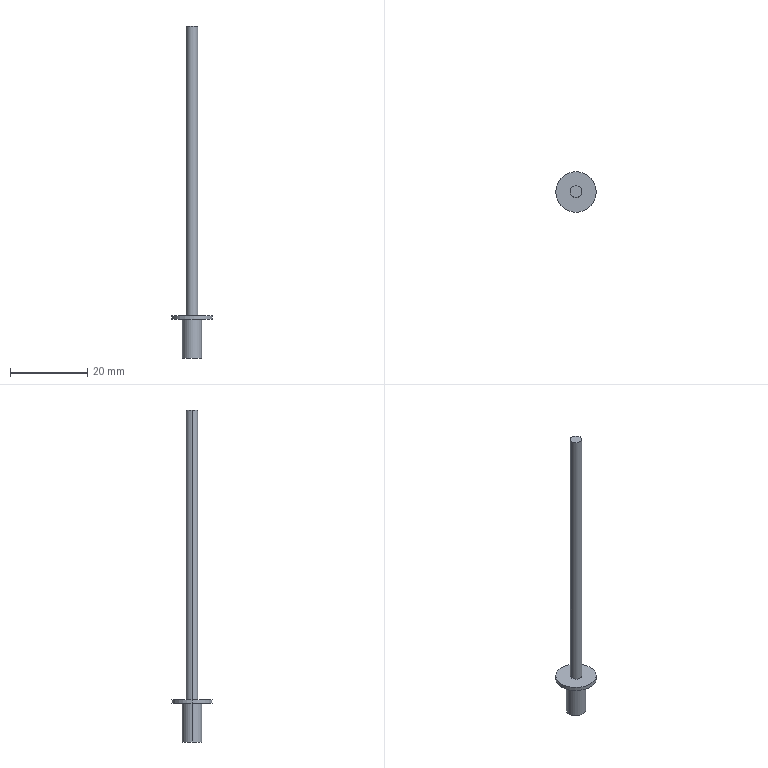Part | Creo | 1 solid | 10 faces | box 10.5 x 10.5 x 86 mm | volume 813.083 mm3 | cylinder 6 | plane 4 | commonest cylinder face diameters 3 x2 5 x2 10.5 x2
STEP:
#1=CARTESIAN_POINT('',(0.,0.,0.));
#2=DIRECTION('',(0.,0.,1.));
#3=DIRECTION('',(1.,0.,0.));
#4=AXIS2_PLACEMENT_3D('',#1,#2,#3);
#5=CARTESIAN_POINT('',(35.5,79.,-54.09));
#6=VERTEX_POINT('',#5);
#7=CARTESIAN_POINT('',(38.5,79.,-54.09));
#8=VERTEX_POINT('',#7);
#9=CARTESIAN_POINT('',(37.,79.,-54.09));
#10=DIRECTION('',(0.,0.,-1.));
#11=DIRECTION('',(-1.,0.,0.));
#12=AXIS2_PLACEMENT_3D('',#9,#10,#11);
#13=CIRCLE('',#12,1.5);
#14=EDGE_CURVE('',#6,#8,#13,.T.);
#15=ORIENTED_EDGE('',*,*,#14,.T.);
#16=CARTESIAN_POINT('',(38.5,79.,20.91));
#17=VERTEX_POINT('',#16);
#18=CARTESIAN_POINT('',(38.5,79.,20.91));
#19=DIRECTION('',(0.,0.,-1.));
#20=VECTOR('',#19,75.);
#21=LINE('',#18,#20);
#22=EDGE_CURVE('',#17,#8,#21,.T.);
#23=ORIENTED_EDGE('',*,*,#22,.F.);
#24=CARTESIAN_POINT('',(35.5,79.,20.91));
#25=VERTEX_POINT('',#24);
#26=CARTESIAN_POINT('',(37.,79.,20.91));
#27=DIRECTION('',(0.,0.,1.));
#28=DIRECTION('',(1.,0.,0.));
#29=AXIS2_PLACEMENT_3D('',#26,#27,#28);
#30=CIRCLE('',#29,1.5);
#31=EDGE_CURVE('',#17,#25,#30,.T.);
#32=ORIENTED_EDGE('',*,*,#31,.T.);
#33=CARTESIAN_POINT('',(35.5,79.,20.91));
#34=DIRECTION('',(0.,0.,-1.));
#35=VECTOR('',#34,75.);
#36=LINE('',#33,#35);
#37=EDGE_CURVE('',#25,#6,#36,.T.);
#38=ORIENTED_EDGE('',*,*,#37,.T.);
#39=EDGE_LOOP('',(#15,#23,#32,#38));
#40=FACE_OUTER_BOUND('',#39,.F.);
#41=CARTESIAN_POINT('',(37.,79.,20.91));
#42=DIRECTION('',(0.,0.,-1.));
#43=DIRECTION('',(-1.,0.,0.));
#44=AXIS2_PLACEMENT_3D('',#41,#42,#43);
#45=CYLINDRICAL_SURFACE('',#44,1.5);
#46=ADVANCED_FACE('',(#40),#45,.T.);
#47=CARTESIAN_POINT('',(31.75,79.,-54.09));
#48=VERTEX_POINT('',#47);
#49=CARTESIAN_POINT('',(42.25,79.,-54.09));
#50=VERTEX_POINT('',#49);
#51=CARTESIAN_POINT('',(37.,79.,-54.09));
#52=DIRECTION('',(0.,0.,1.));
#53=DIRECTION('',(-1.,0.,0.));
#54=AXIS2_PLACEMENT_3D('',#51,#52,#53);
#55=CIRCLE('',#54,5.25);
#56=EDGE_CURVE('',#48,#50,#55,.T.);
#57=ORIENTED_EDGE('',*,*,#56,.F.);
#58=CARTESIAN_POINT('',(37.,79.,-54.09));
#59=DIRECTION('',(0.,0.,1.));
#60=DIRECTION('',(1.,0.,0.));
#61=AXIS2_PLACEMENT_3D('',#58,#59,#60);
#62=CIRCLE('',#61,5.25);
#63=EDGE_CURVE('',#50,#48,#62,.T.);
#64=ORIENTED_EDGE('',*,*,#63,.F.);
#65=EDGE_LOOP('',(#57,#64));
#66=FACE_OUTER_BOUND('',#65,.F.);
#67=ORIENTED_EDGE('',*,*,#14,.F.);
#68=CARTESIAN_POINT('',(37.,79.,-54.09));
#69=DIRECTION('',(0.,0.,-1.));
#70=DIRECTION('',(1.,0.,0.));
#71=AXIS2_PLACEMENT_3D('',#68,#69,#70);
#72=CIRCLE('',#71,1.5);
#73=EDGE_CURVE('',#8,#6,#72,.T.);
#74=ORIENTED_EDGE('',*,*,#73,.F.);
#75=EDGE_LOOP('',(#67,#74));
#76=FACE_BOUND('',#75,.F.);
#77=CARTESIAN_POINT('',(0.,0.,-54.09));
#78=DIRECTION('',(0.,0.,-1.));
#79=DIRECTION('',(-1.,0.,0.));
#80=AXIS2_PLACEMENT_3D('',#77,#78,#79);
#81=PLANE('',#80);
#82=ADVANCED_FACE('',(#66,#76),#81,.F.);
#83=ORIENTED_EDGE('',*,*,#73,.T.);
#84=ORIENTED_EDGE('',*,*,#37,.F.);
#85=CARTESIAN_POINT('',(37.,79.,20.91));
#86=DIRECTION('',(0.,0.,1.));
#87=DIRECTION('',(-1.,0.,0.));
#88=AXIS2_PLACEMENT_3D('',#85,#86,#87);
#89=CIRCLE('',#88,1.5);
#90=EDGE_CURVE('',#25,#17,#89,.T.);
#91=ORIENTED_EDGE('',*,*,#90,.T.);
#92=ORIENTED_EDGE('',*,*,#22,.T.);
#93=EDGE_LOOP('',(#83,#84,#91,#92));
#94=FACE_OUTER_BOUND('',#93,.F.);
#95=CARTESIAN_POINT('',(37.,79.,20.91));
#96=DIRECTION('',(0.,0.,-1.));
#97=DIRECTION('',(-1.,0.,0.));
#98=AXIS2_PLACEMENT_3D('',#95,#96,#97);
#99=CYLINDRICAL_SURFACE('',#98,1.5);
#100=ADVANCED_FACE('',(#94),#99,.T.);
#101=ORIENTED_EDGE('',*,*,#90,.F.);
#102=ORIENTED_EDGE('',*,*,#31,.F.);
#103=EDGE_LOOP('',(#101,#102));
#104=FACE_OUTER_BOUND('',#103,.F.);
#105=CARTESIAN_POINT('',(37.,79.,20.91));
#106=DIRECTION('',(0.,0.,-1.));
#107=DIRECTION('',(-1.,0.,0.));
#108=AXIS2_PLACEMENT_3D('',#105,#106,#107);
#109=PLANE('',#108);
#110=ADVANCED_FACE('',(#104),#109,.F.);
#111=ORIENTED_EDGE('',*,*,#56,.T.);
#112=CARTESIAN_POINT('',(42.25,79.,-55.09));
#113=VERTEX_POINT('',#112);
#114=CARTESIAN_POINT('',(42.25,79.,-55.09));
#115=DIRECTION('',(0.,0.,1.));
#116=VECTOR('',#115,1.);
#117=LINE('',#114,#116);
#118=EDGE_CURVE('',#113,#50,#117,.T.);
#119=ORIENTED_EDGE('',*,*,#118,.F.);
#120=CARTESIAN_POINT('',(31.75,79.,-55.09));
#121=VERTEX_POINT('',#120);
#122=CARTESIAN_POINT('',(37.,79.,-55.09));
#123=DIRECTION('',(0.,0.,-1.));
#124=DIRECTION('',(1.,0.,0.));
#125=AXIS2_PLACEMENT_3D('',#122,#123,#124);
#126=CIRCLE('',#125,5.25);
#127=EDGE_CURVE('',#113,#121,#126,.T.);
#128=ORIENTED_EDGE('',*,*,#127,.T.);
#129=CARTESIAN_POINT('',(31.75,79.,-55.09));
#130=DIRECTION('',(0.,0.,1.));
#131=VECTOR('',#130,1.);
#132=LINE('',#129,#131);
#133=EDGE_CURVE('',#121,#48,#132,.T.);
#134=ORIENTED_EDGE('',*,*,#133,.T.);
#135=EDGE_LOOP('',(#111,#119,#128,#134));
#136=FACE_OUTER_BOUND('',#135,.F.);
#137=CARTESIAN_POINT('',(37.,79.,-104.09));
#138=DIRECTION('',(0.,0.,1.));
#139=DIRECTION('',(1.,0.,0.));
#140=AXIS2_PLACEMENT_3D('',#137,#138,#139);
#141=CYLINDRICAL_SURFACE('',#140,5.25);
#142=ADVANCED_FACE('',(#136),#141,.T.);
#143=ORIENTED_EDGE('',*,*,#63,.T.);
#144=ORIENTED_EDGE('',*,*,#133,.F.);
#145=CARTESIAN_POINT('',(37.,79.,-55.09));
#146=DIRECTION('',(0.,0.,-1.));
#147=DIRECTION('',(-1.,0.,0.));
#148=AXIS2_PLACEMENT_3D('',#145,#146,#147);
#149=CIRCLE('',#148,5.25);
#150=EDGE_CURVE('',#121,#113,#149,.T.);
#151=ORIENTED_EDGE('',*,*,#150,.T.);
#152=ORIENTED_EDGE('',*,*,#118,.T.);
#153=EDGE_LOOP('',(#143,#144,#151,#152));
#154=FACE_OUTER_BOUND('',#153,.F.);
#155=CARTESIAN_POINT('',(37.,79.,-104.09));
#156=DIRECTION('',(0.,0.,1.));
#157=DIRECTION('',(1.,0.,0.));
#158=AXIS2_PLACEMENT_3D('',#155,#156,#157);
#159=CYLINDRICAL_SURFACE('',#158,5.25);
#160=ADVANCED_FACE('',(#154),#159,.T.);
#161=ORIENTED_EDGE('',*,*,#150,.F.);
#162=ORIENTED_EDGE('',*,*,#127,.F.);
#163=EDGE_LOOP('',(#161,#162));
#164=FACE_OUTER_BOUND('',#163,.F.);
#165=CARTESIAN_POINT('',(34.5,79.,-55.09));
#166=VERTEX_POINT('',#165);
#167=CARTESIAN_POINT('',(39.5,79.,-55.09));
#168=VERTEX_POINT('',#167);
#169=CARTESIAN_POINT('',(37.,79.,-55.09));
#170=DIRECTION('',(0.,0.,1.));
#171=DIRECTION('',(-1.,0.,0.));
#172=AXIS2_PLACEMENT_3D('',#169,#170,#171);
#173=CIRCLE('',#172,2.5);
#174=EDGE_CURVE('',#166,#168,#173,.T.);
#175=ORIENTED_EDGE('',*,*,#174,.F.);
#176=CARTESIAN_POINT('',(37.,79.,-55.09));
#177=DIRECTION('',(0.,0.,1.));
#178=DIRECTION('',(1.,0.,0.));
#179=AXIS2_PLACEMENT_3D('',#176,#177,#178);
#180=CIRCLE('',#179,2.5);
#181=EDGE_CURVE('',#168,#166,#180,.T.);
#182=ORIENTED_EDGE('',*,*,#181,.F.);
#183=EDGE_LOOP('',(#175,#182));
#184=FACE_BOUND('',#183,.F.);
#185=CARTESIAN_POINT('',(0.,0.,-55.09));
#186=DIRECTION('',(0.,0.,-1.));
#187=DIRECTION('',(-1.,0.,0.));
#188=AXIS2_PLACEMENT_3D('',#185,#186,#187);
#189=PLANE('',#188);
#190=ADVANCED_FACE('',(#164,#184),#189,.T.);
#191=CARTESIAN_POINT('',(39.5,79.,-65.09));
#192=VERTEX_POINT('',#191);
#193=CARTESIAN_POINT('',(34.5,79.,-65.09));
#194=VERTEX_POINT('',#193);
#195=CARTESIAN_POINT('',(37.,79.,-65.09));
#196=DIRECTION('',(0.,0.,-1.));
#197=DIRECTION('',(1.,0.,0.));
#198=AXIS2_PLACEMENT_3D('',#195,#196,#197);
#199=CIRCLE('',#198,2.5);
#200=EDGE_CURVE('',#192,#194,#199,.T.);
#201=ORIENTED_EDGE('',*,*,#200,.T.);
#202=CARTESIAN_POINT('',(34.5,79.,-55.09));
#203=DIRECTION('',(0.,0.,-1.));
#204=VECTOR('',#203,10.);
#205=LINE('',#202,#204);
#206=EDGE_CURVE('',#166,#194,#205,.T.);
#207=ORIENTED_EDGE('',*,*,#206,.F.);
#208=ORIENTED_EDGE('',*,*,#174,.T.);
#209=CARTESIAN_POINT('',(39.5,79.,-55.09));
#210=DIRECTION('',(0.,0.,-1.));
#211=VECTOR('',#210,10.);
#212=LINE('',#209,#211);
#213=EDGE_CURVE('',#168,#192,#212,.T.);
#214=ORIENTED_EDGE('',*,*,#213,.T.);
#215=EDGE_LOOP('',(#201,#207,#208,#214));
#216=FACE_OUTER_BOUND('',#215,.F.);
#217=CARTESIAN_POINT('',(37.,79.,-55.09));
#218=DIRECTION('',(0.,0.,-1.));
#219=DIRECTION('',(-1.,0.,0.));
#220=AXIS2_PLACEMENT_3D('',#217,#218,#219);
#221=CYLINDRICAL_SURFACE('',#220,2.5);
#222=ADVANCED_FACE('',(#216),#221,.T.);
#223=ORIENTED_EDGE('',*,*,#200,.F.);
#224=CARTESIAN_POINT('',(37.,79.,-65.09));
#225=DIRECTION('',(0.,0.,-1.));
#226=DIRECTION('',(-1.,0.,0.));
#227=AXIS2_PLACEMENT_3D('',#224,#225,#226);
#228=CIRCLE('',#227,2.5);
#229=EDGE_CURVE('',#194,#192,#228,.T.);
#230=ORIENTED_EDGE('',*,*,#229,.F.);
#231=EDGE_LOOP('',(#223,#230));
#232=FACE_OUTER_BOUND('',#231,.F.);
#233=CARTESIAN_POINT('',(37.,79.,-65.09));
#234=DIRECTION('',(0.,0.,1.));
#235=DIRECTION('',(1.,0.,0.));
#236=AXIS2_PLACEMENT_3D('',#233,#234,#235);
#237=PLANE('',#236);
#238=ADVANCED_FACE('',(#232),#237,.F.);
#239=ORIENTED_EDGE('',*,*,#229,.T.);
#240=ORIENTED_EDGE('',*,*,#213,.F.);
#241=ORIENTED_EDGE('',*,*,#181,.T.);
#242=ORIENTED_EDGE('',*,*,#206,.T.);
#243=EDGE_LOOP('',(#239,#240,#241,#242));
#244=FACE_OUTER_BOUND('',#243,.F.);
#245=CARTESIAN_POINT('',(37.,79.,-55.09));
#246=DIRECTION('',(0.,0.,-1.));
#247=DIRECTION('',(-1.,0.,0.));
#248=AXIS2_PLACEMENT_3D('',#245,#246,#247);
#249=CYLINDRICAL_SURFACE('',#248,2.5);
#250=ADVANCED_FACE('',(#244),#249,.T.);
#251=CLOSED_SHELL('',(#46,#82,#100,#110,#142,#160,#190,#222,#238,#250));
#252=MANIFOLD_SOLID_BREP('',#251);
#253=(LENGTH_UNIT()NAMED_UNIT(*)SI_UNIT(.MILLI.,.METRE.));
#254=UNCERTAINTY_MEASURE_WITH_UNIT(LENGTH_MEASURE(0.008727),#253,'','');
#255=(NAMED_UNIT(*)PLANE_ANGLE_UNIT()SI_UNIT($,.RADIAN.));
#256=PLANE_ANGLE_MEASURE_WITH_UNIT(PLANE_ANGLE_MEASURE(0.01745),#255);
#257=(CONVERSION_BASED_UNIT('DEGREE',#256)NAMED_UNIT(*)PLANE_ANGLE_UNIT());
#258=(NAMED_UNIT(*)SI_UNIT($,.STERADIAN.)SOLID_ANGLE_UNIT());
#259=(GEOMETRIC_REPRESENTATION_CONTEXT(3)GLOBAL_UNCERTAINTY_ASSIGNED_CONTEXT((#254))GLOBAL_UNIT_ASSIGNED_CONTEXT((#253,#257,#258))REPRESENTATION_CONTEXT('',''));
#260=ADVANCED_BREP_SHAPE_REPRESENTATION('',(#4,#252),#259);